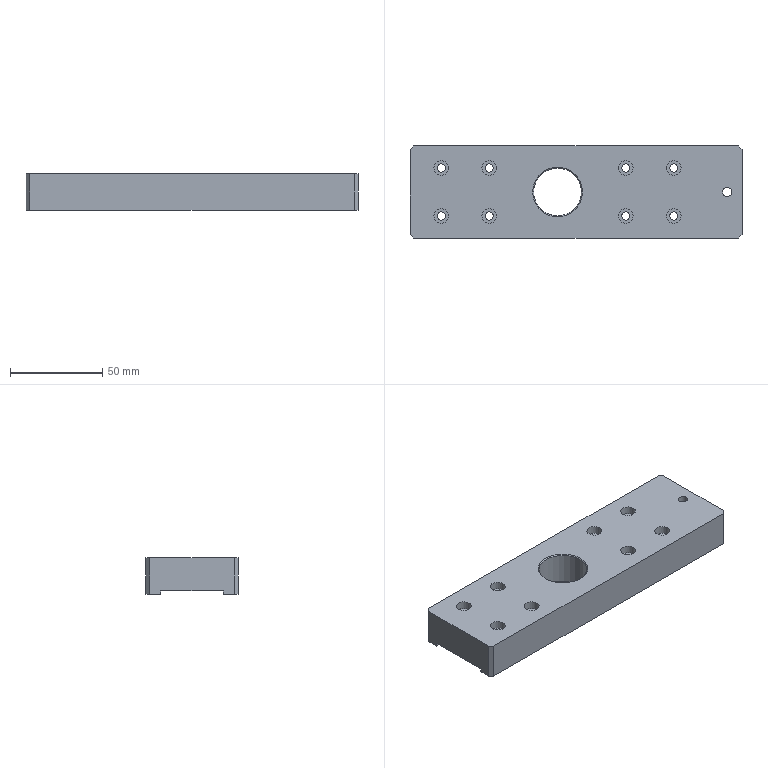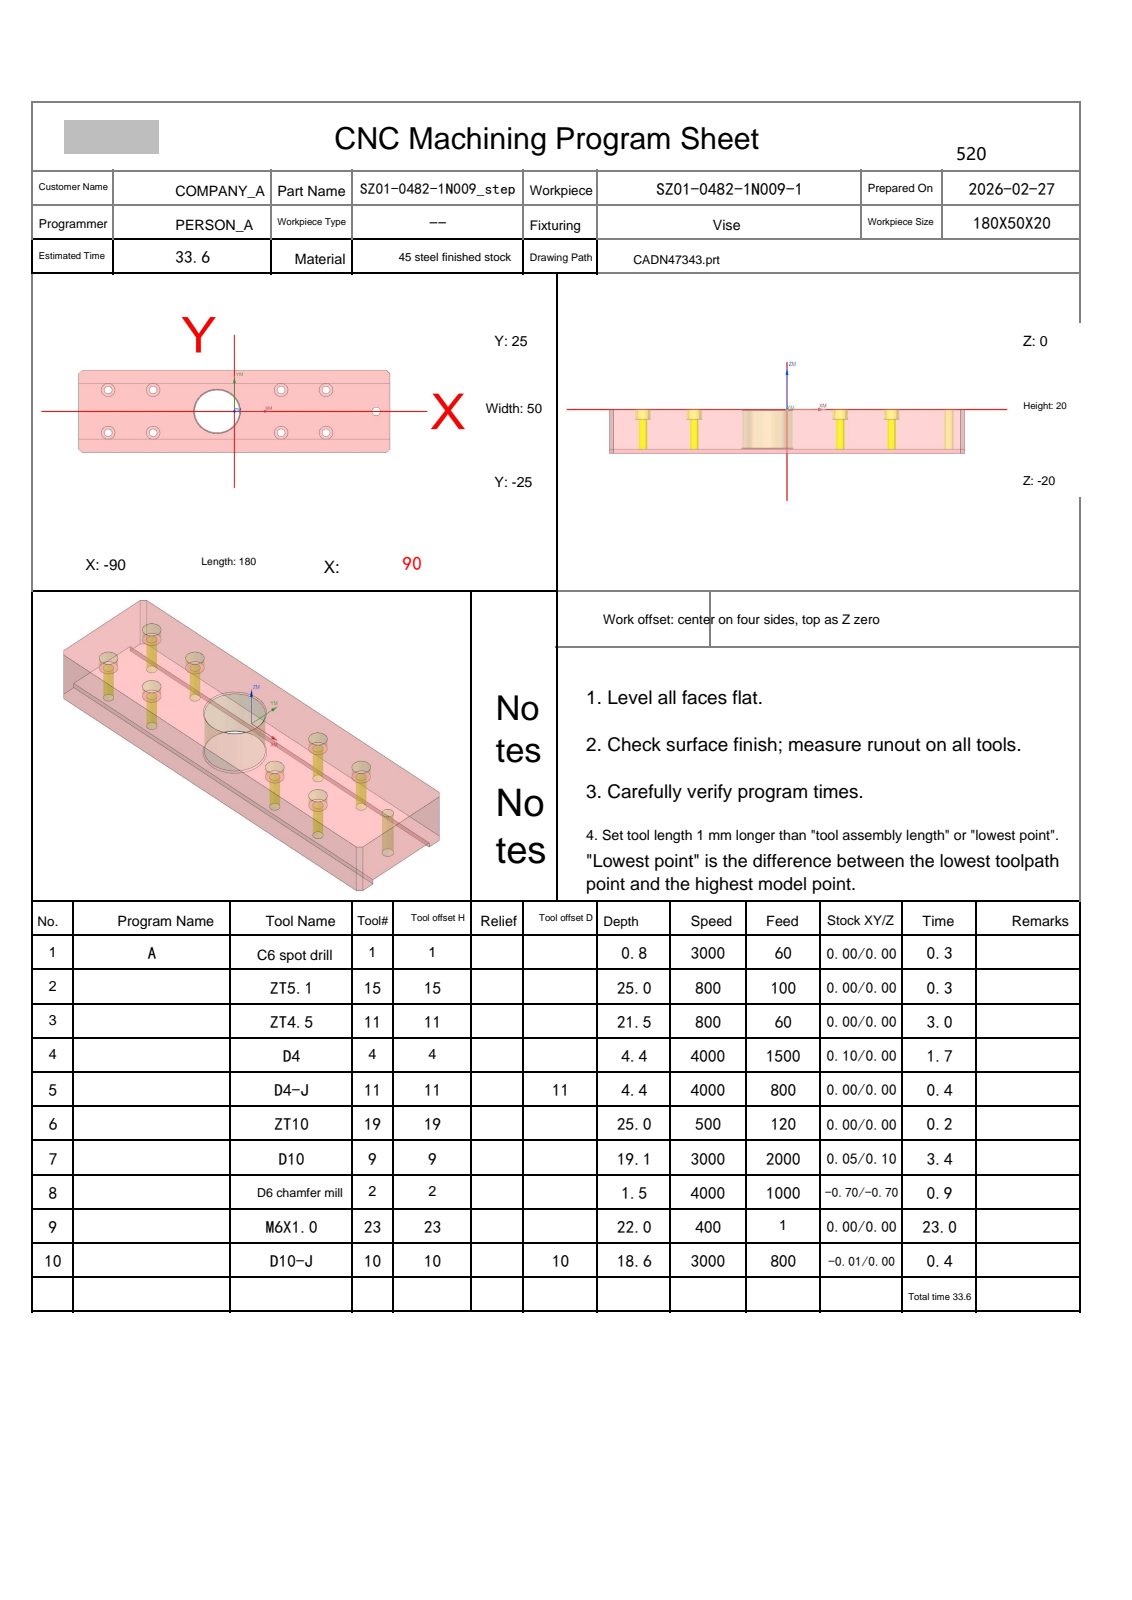NC program | NX | posted by the shop | part box 180 x 50 x 20 mm
Whole program, first 1459 of 1632 lines:
%
O0001
(Machine time: 57.60 MIN)
(===Total Tool:9===)
(T1=C6 spot drill   D=6.   R=0.   D-  H01 Z=-0.8  )
(T15=ZT5.1  D=5.1  DR_a=118 D-  H15 Z=-25.  )
(T11=ZT4.5  D=4.5  DR_a=118 D-  H11 Z=-21.45)
(T4=D4      D=4.   R=0.   D-  H04 Z=-4.4  )
(T19=ZT10   D=10.  DR_a=118 D-  H19 Z=-25.  )
(T9=D10     D=10.  R=0.   D-  H09 Z=-19.1 )
(T2=D6 chamfer mill   D=6.   R=0.   D-  H02 Z=-1.5  )
(T23=M6X1.0 D=5.   DR_a=180 D-  H23 Z=-22.  )
(T10=D10-J  D=10.  R=0.   D10 H10 Z=-18.6 )
G80 G90 G17 G49 G40
G91 G28 Z0
M01
N1 T01 M06
(C6 spot drill  D=6. R=0. H=01 ce=0.00 di=0.00)
T15
G00 G90 G54 X-47. Y13. M03 S3000
G43 H01 Z30.
M08
G98 G81 X-47. Y13. Z-.8 R1. F60.
X-73.
Y-13.
X-47.
X-10. Y0.0
X27. Y-13.
Y13.
X53.
Y-13.
X82. Y0.0
G80
G00 Z30.
G91 G28 Z0.0
M05
M09
G91 G28 Z0.0
M01
N2 T15 M06
(ZT5.1 D=5.1 DR_a=118 H=15)
T11
G00 G90 G54 X82. Y0.0 M03 S800
G43 H15 Z30.
M08
G98 G83 X82. Y0.0 Z-25. R1. F100. Q2.
G80
G00 Z30.
G91 G28 Z0.0
M05
M09
G91 G28 Z0.0
M01
N3 T11 M06
(ZT4.5 D=4.5 DR_a=118 H=11)
T04
G00 G90 G54 X-47. Y-13. M03 S800
G43 H11 Z30.
M08
G98 G83 X-47. Y-13. Z-21.452 R1. F60. Q1.
X-73.
Y13.
X-47.
X27.
Y-13.
X53.
Y13.
G80
G00 Z30.
G91 G28 Z0.0
M05
M09
G91 G28 Z0.0
M01
N4 T04 M06
(D4  D=4. R=0. H=04 ce=0.10 di=0.00)
T11
G00 G90 G54 X-73. Y-13. M03 S4000
G43 H04 Z30.
M08
Z.5
G03 X-72.05 Y-13.95 I.95 J0.0 F1500.
X-71.1 Y-13. I0.0 J.95
X-71.1 Y-13. Z.3 I-1.9 J0.0
X-71.1 Y-13. Z.1 I-1.9 J0.0
X-71.1 Y-13. Z-.1 I-1.9 J0.0
X-71.1 Y-13. Z-.3 I-1.9 J0.0
X-71.1 Y-13. Z-.5 I-1.9 J0.0
X-71.1 Y-13. Z-.7 I-1.9 J0.0
X-71.1 Y-13. Z-.9 I-1.9 J0.0
X-71.1 Y-13. Z-1.1 I-1.9 J0.0
X-71.1 Y-13. Z-1.3 I-1.9 J0.0
X-71.1 Y-13. Z-1.5 I-1.9 J0.0
X-71.1 Y-13. Z-1.7 I-1.9 J0.0
X-71.1 Y-13. Z-1.9 I-1.9 J0.0
X-71.1 Y-13. Z-2.1 I-1.9 J0.0
X-71.1 Y-13. Z-2.3 I-1.9 J0.0
X-71.1 Y-13. Z-2.5 I-1.9 J0.0
X-71.1 Y-13. Z-2.7 I-1.9 J0.0
X-71.1 Y-13. Z-2.9 I-1.9 J0.0
X-71.1 Y-13. Z-3.1 I-1.9 J0.0
X-71.1 Y-13. Z-3.3 I-1.9 J0.0
X-71.1 Y-13. Z-3.5 I-1.9 J0.0
X-71.1 Y-13. Z-3.7 I-1.9 J0.0
X-71.1 Y-13. Z-3.9 I-1.9 J0.0
X-71.1 Y-13. Z-4.1 I-1.9 J0.0
X-71.1 Y-13. Z-4.3 I-1.9 J0.0
X-74.9 Y-13. Z-4.4 I-1.9 J0.0
X-73. Y-14.9 I1.9 J0.0
X-71.1 Y-13. I0.0 J1.9
X-73. Y-11.1 I-1.9 J0.0
X-74.9 Y-13. I0.0 J-1.9
X-73.95 Y-13.95 I.95 J0.0
X-73. Y-13. I0.0 J.95
G00 Z30.
Y13.
Z.5
G03 X-72.05 Y12.05 I.95 J0.0
X-71.1 Y13. I0.0 J.95
X-71.1 Y13. Z.3 I-1.9 J0.0
X-71.1 Y13. Z.1 I-1.9 J0.0
X-71.1 Y13. Z-.1 I-1.9 J0.0
X-71.1 Y13. Z-.3 I-1.9 J0.0
X-71.1 Y13. Z-.5 I-1.9 J0.0
X-71.1 Y13. Z-.7 I-1.9 J0.0
X-71.1 Y13. Z-.9 I-1.9 J0.0
X-71.1 Y13. Z-1.1 I-1.9 J0.0
X-71.1 Y13. Z-1.3 I-1.9 J0.0
X-71.1 Y13. Z-1.5 I-1.9 J0.0
X-71.1 Y13. Z-1.7 I-1.9 J0.0
X-71.1 Y13. Z-1.9 I-1.9 J0.0
X-71.1 Y13. Z-2.1 I-1.9 J0.0
X-71.1 Y13. Z-2.3 I-1.9 J0.0
X-71.1 Y13. Z-2.5 I-1.9 J0.0
X-71.1 Y13. Z-2.7 I-1.9 J0.0
X-71.1 Y13. Z-2.9 I-1.9 J0.0
X-71.1 Y13. Z-3.1 I-1.9 J0.0
X-71.1 Y13. Z-3.3 I-1.9 J0.0
X-71.1 Y13. Z-3.5 I-1.9 J0.0
X-71.1 Y13. Z-3.7 I-1.9 J0.0
X-71.1 Y13. Z-3.9 I-1.9 J0.0
X-71.1 Y13. Z-4.1 I-1.9 J0.0
X-71.1 Y13. Z-4.3 I-1.9 J0.0
X-74.9 Y13. Z-4.4 I-1.9 J0.0
X-73. Y11.1 I1.9 J0.0
X-71.1 Y13. I0.0 J1.9
X-73. Y14.9 I-1.9 J0.0
X-74.9 Y13. I0.0 J-1.9
X-73.95 Y12.05 I.95 J0.0
X-73. Y13. I0.0 J.95
G00 Z30.
X-47.
Z.5
G03 X-46.05 Y12.05 I.95 J0.0
X-45.1 Y13. I0.0 J.95
X-45.1 Y13. Z.3 I-1.9 J0.0
X-45.1 Y13. Z.1 I-1.9 J0.0
X-45.1 Y13. Z-.1 I-1.9 J0.0
X-45.1 Y13. Z-.3 I-1.9 J0.0
X-45.1 Y13. Z-.5 I-1.9 J0.0
X-45.1 Y13. Z-.7 I-1.9 J0.0
X-45.1 Y13. Z-.9 I-1.9 J0.0
X-45.1 Y13. Z-1.1 I-1.9 J0.0
X-45.1 Y13. Z-1.3 I-1.9 J0.0
X-45.1 Y13. Z-1.5 I-1.9 J0.0
X-45.1 Y13. Z-1.7 I-1.9 J0.0
X-45.1 Y13. Z-1.9 I-1.9 J0.0
X-45.1 Y13. Z-2.1 I-1.9 J0.0
X-45.1 Y13. Z-2.3 I-1.9 J0.0
X-45.1 Y13. Z-2.5 I-1.9 J0.0
X-45.1 Y13. Z-2.7 I-1.9 J0.0
X-45.1 Y13. Z-2.9 I-1.9 J0.0
X-45.1 Y13. Z-3.1 I-1.9 J0.0
X-45.1 Y13. Z-3.3 I-1.9 J0.0
X-45.1 Y13. Z-3.5 I-1.9 J0.0
X-45.1 Y13. Z-3.7 I-1.9 J0.0
X-45.1 Y13. Z-3.9 I-1.9 J0.0
X-45.1 Y13. Z-4.1 I-1.9 J0.0
X-45.1 Y13. Z-4.3 I-1.9 J0.0
X-48.9 Y13. Z-4.4 I-1.9 J0.0
X-47. Y11.1 I1.9 J0.0
X-45.1 Y13. I0.0 J1.9
X-47. Y14.9 I-1.9 J0.0
X-48.9 Y13. I0.0 J-1.9
X-47.95 Y12.05 I.95 J0.0
X-47. Y13. I0.0 J.95
G00 Z30.
Y-13.
Z.5
G03 X-46.05 Y-13.95 I.95 J0.0
X-45.1 Y-13. I0.0 J.95
X-45.1 Y-13. Z.3 I-1.9 J0.0
X-45.1 Y-13. Z.1 I-1.9 J0.0
X-45.1 Y-13. Z-.1 I-1.9 J0.0
X-45.1 Y-13. Z-.3 I-1.9 J0.0
X-45.1 Y-13. Z-.5 I-1.9 J0.0
X-45.1 Y-13. Z-.7 I-1.9 J0.0
X-45.1 Y-13. Z-.9 I-1.9 J0.0
X-45.1 Y-13. Z-1.1 I-1.9 J0.0
X-45.1 Y-13. Z-1.3 I-1.9 J0.0
X-45.1 Y-13. Z-1.5 I-1.9 J0.0
X-45.1 Y-13. Z-1.7 I-1.9 J0.0
X-45.1 Y-13. Z-1.9 I-1.9 J0.0
X-45.1 Y-13. Z-2.1 I-1.9 J0.0
X-45.1 Y-13. Z-2.3 I-1.9 J0.0
X-45.1 Y-13. Z-2.5 I-1.9 J0.0
X-45.1 Y-13. Z-2.7 I-1.9 J0.0
X-45.1 Y-13. Z-2.9 I-1.9 J0.0
X-45.1 Y-13. Z-3.1 I-1.9 J0.0
X-45.1 Y-13. Z-3.3 I-1.9 J0.0
X-45.1 Y-13. Z-3.5 I-1.9 J0.0
X-45.1 Y-13. Z-3.7 I-1.9 J0.0
X-45.1 Y-13. Z-3.9 I-1.9 J0.0
X-45.1 Y-13. Z-4.1 I-1.9 J0.0
X-45.1 Y-13. Z-4.3 I-1.9 J0.0
X-48.9 Y-13. Z-4.4 I-1.9 J0.0
X-47. Y-14.9 I1.9 J0.0
X-45.1 Y-13. I0.0 J1.9
X-47. Y-11.1 I-1.9 J0.0
X-48.9 Y-13. I0.0 J-1.9
X-47.95 Y-13.95 I.95 J0.0
X-47. Y-13. I0.0 J.95
G00 Z30.
X27.
Z.5
G03 X27.95 Y-13.95 I.95 J0.0
X28.9 Y-13. I0.0 J.95
X28.9 Y-13. Z.3 I-1.9 J0.0
X28.9 Y-13. Z.1 I-1.9 J0.0
X28.9 Y-13. Z-.1 I-1.9 J0.0
X28.9 Y-13. Z-.3 I-1.9 J0.0
X28.9 Y-13. Z-.5 I-1.9 J0.0
X28.9 Y-13. Z-.7 I-1.9 J0.0
X28.9 Y-13. Z-.9 I-1.9 J0.0
X28.9 Y-13. Z-1.1 I-1.9 J0.0
X28.9 Y-13. Z-1.3 I-1.9 J0.0
X28.9 Y-13. Z-1.5 I-1.9 J0.0
X28.9 Y-13. Z-1.7 I-1.9 J0.0
X28.9 Y-13. Z-1.9 I-1.9 J0.0
X28.9 Y-13. Z-2.1 I-1.9 J0.0
X28.9 Y-13. Z-2.3 I-1.9 J0.0
X28.9 Y-13. Z-2.5 I-1.9 J0.0
X28.9 Y-13. Z-2.7 I-1.9 J0.0
X28.9 Y-13. Z-2.9 I-1.9 J0.0
X28.9 Y-13. Z-3.1 I-1.9 J0.0
X28.9 Y-13. Z-3.3 I-1.9 J0.0
X28.9 Y-13. Z-3.5 I-1.9 J0.0
X28.9 Y-13. Z-3.7 I-1.9 J0.0
X28.9 Y-13. Z-3.9 I-1.9 J0.0
X28.9 Y-13. Z-4.1 I-1.9 J0.0
X28.9 Y-13. Z-4.3 I-1.9 J0.0
X25.1 Y-13. Z-4.4 I-1.9 J0.0
X27. Y-14.9 I1.9 J0.0
X28.9 Y-13. I0.0 J1.9
X27. Y-11.1 I-1.9 J0.0
X25.1 Y-13. I0.0 J-1.9
X26.05 Y-13.95 I.95 J0.0
X27. Y-13. I0.0 J.95
G00 Z30.
X53.
Z.5
G03 X53.95 Y-13.95 I.95 J0.0
X54.9 Y-13. I0.0 J.95
X54.9 Y-13. Z.3 I-1.9 J0.0
X54.9 Y-13. Z.1 I-1.9 J0.0
X54.9 Y-13. Z-.1 I-1.9 J0.0
X54.9 Y-13. Z-.3 I-1.9 J0.0
X54.9 Y-13. Z-.5 I-1.9 J0.0
X54.9 Y-13. Z-.7 I-1.9 J0.0
X54.9 Y-13. Z-.9 I-1.9 J0.0
X54.9 Y-13. Z-1.1 I-1.9 J0.0
X54.9 Y-13. Z-1.3 I-1.9 J0.0
X54.9 Y-13. Z-1.5 I-1.9 J0.0
X54.9 Y-13. Z-1.7 I-1.9 J0.0
X54.9 Y-13. Z-1.9 I-1.9 J0.0
X54.9 Y-13. Z-2.1 I-1.9 J0.0
X54.9 Y-13. Z-2.3 I-1.9 J0.0
X54.9 Y-13. Z-2.5 I-1.9 J0.0
X54.9 Y-13. Z-2.7 I-1.9 J0.0
X54.9 Y-13. Z-2.9 I-1.9 J0.0
X54.9 Y-13. Z-3.1 I-1.9 J0.0
X54.9 Y-13. Z-3.3 I-1.9 J0.0
X54.9 Y-13. Z-3.5 I-1.9 J0.0
X54.9 Y-13. Z-3.7 I-1.9 J0.0
X54.9 Y-13. Z-3.9 I-1.9 J0.0
X54.9 Y-13. Z-4.1 I-1.9 J0.0
X54.9 Y-13. Z-4.3 I-1.9 J0.0
X51.1 Y-13. Z-4.4 I-1.9 J0.0
X53. Y-14.9 I1.9 J0.0
X54.9 Y-13. I0.0 J1.9
X53. Y-11.1 I-1.9 J0.0
X51.1 Y-13. I0.0 J-1.9
X52.05 Y-13.95 I.95 J0.0
X53. Y-13. I0.0 J.95
G00 Z30.
Y13.
Z.5
G03 X53.95 Y12.05 I.95 J0.0
X54.9 Y13. I0.0 J.95
X54.9 Y13. Z.3 I-1.9 J0.0
X54.9 Y13. Z.1 I-1.9 J0.0
X54.9 Y13. Z-.1 I-1.9 J0.0
X54.9 Y13. Z-.3 I-1.9 J0.0
X54.9 Y13. Z-.5 I-1.9 J0.0
X54.9 Y13. Z-.7 I-1.9 J0.0
X54.9 Y13. Z-.9 I-1.9 J0.0
X54.9 Y13. Z-1.1 I-1.9 J0.0
X54.9 Y13. Z-1.3 I-1.9 J0.0
X54.9 Y13. Z-1.5 I-1.9 J0.0
X54.9 Y13. Z-1.7 I-1.9 J0.0
X54.9 Y13. Z-1.9 I-1.9 J0.0
X54.9 Y13. Z-2.1 I-1.9 J0.0
X54.9 Y13. Z-2.3 I-1.9 J0.0
X54.9 Y13. Z-2.5 I-1.9 J0.0
X54.9 Y13. Z-2.7 I-1.9 J0.0
X54.9 Y13. Z-2.9 I-1.9 J0.0
X54.9 Y13. Z-3.1 I-1.9 J0.0
X54.9 Y13. Z-3.3 I-1.9 J0.0
X54.9 Y13. Z-3.5 I-1.9 J0.0
X54.9 Y13. Z-3.7 I-1.9 J0.0
X54.9 Y13. Z-3.9 I-1.9 J0.0
X54.9 Y13. Z-4.1 I-1.9 J0.0
X54.9 Y13. Z-4.3 I-1.9 J0.0
X51.1 Y13. Z-4.4 I-1.9 J0.0
X53. Y11.1 I1.9 J0.0
X54.9 Y13. I0.0 J1.9
X53. Y14.9 I-1.9 J0.0
X51.1 Y13. I0.0 J-1.9
X52.05 Y12.05 I.95 J0.0
X53. Y13. I0.0 J.95
G00 Z30.
X27.
Z.5
G03 X27.95 Y12.05 I.95 J0.0
X28.9 Y13. I0.0 J.95
X28.9 Y13. Z.3 I-1.9 J0.0
X28.9 Y13. Z.1 I-1.9 J0.0
X28.9 Y13. Z-.1 I-1.9 J0.0
X28.9 Y13. Z-.3 I-1.9 J0.0
X28.9 Y13. Z-.5 I-1.9 J0.0
X28.9 Y13. Z-.7 I-1.9 J0.0
X28.9 Y13. Z-.9 I-1.9 J0.0
X28.9 Y13. Z-1.1 I-1.9 J0.0
X28.9 Y13. Z-1.3 I-1.9 J0.0
X28.9 Y13. Z-1.5 I-1.9 J0.0
X28.9 Y13. Z-1.7 I-1.9 J0.0
X28.9 Y13. Z-1.9 I-1.9 J0.0
X28.9 Y13. Z-2.1 I-1.9 J0.0
X28.9 Y13. Z-2.3 I-1.9 J0.0
X28.9 Y13. Z-2.5 I-1.9 J0.0
X28.9 Y13. Z-2.7 I-1.9 J0.0
X28.9 Y13. Z-2.9 I-1.9 J0.0
X28.9 Y13. Z-3.1 I-1.9 J0.0
X28.9 Y13. Z-3.3 I-1.9 J0.0
X28.9 Y13. Z-3.5 I-1.9 J0.0
X28.9 Y13. Z-3.7 I-1.9 J0.0
X28.9 Y13. Z-3.9 I-1.9 J0.0
X28.9 Y13. Z-4.1 I-1.9 J0.0
X28.9 Y13. Z-4.3 I-1.9 J0.0
X25.1 Y13. Z-4.4 I-1.9 J0.0
X27. Y11.1 I1.9 J0.0
X28.9 Y13. I0.0 J1.9
X27. Y14.9 I-1.9 J0.0
X25.1 Y13. I0.0 J-1.9
X26.05 Y12.05 I.95 J0.0
X27. Y13. I0.0 J.95
G00 Z30.
G91 G28 Z0.0
M05
M09
G91 G28 Z0.0
M01
N5 T11 M06
(D4-J  D=4. R=0. H=11 ce=0.00 di=0.00)
T19
G00 G90 G54 X-73. Y-13. M03 S4000
G43 H11 Z30.
M08
Z.5
G41 D11
G01 X-72.96 Y-13.196 F800.
G03 X-71.99 Y-13.99 I.97 J.196
X-71. Y-13. I0.0 J.99
X-71.016 Y-13.251 Z-4.4 I-2. J0.0
X-71. Y-13. I-1.984 J.251
X-73. Y-11. I-2. J0.0
X-75. Y-13. I0.0 J-2.
X-73. Y-15. I2. J0.0
X-71.016 Y-13.251 I0.0 J2.
G01 X-71.008 Y-13.127
G03 X-71.998 Y-12.137 I-.99 J0.0
X-72.936 Y-12.81 I0.0 J-.99
G01 G40 X-73. Y-13.
G00 Z30.
Y13.
Z.5
G41 D11
G01 X-72.96 Y12.804
G03 X-71.99 Y12.01 I.97 J.196
X-71. Y13. I0.0 J.99
X-71.016 Y12.749 Z-4.4 I-2. J0.0
X-71. Y13. I-1.984 J.251
X-73. Y15. I-2. J0.0
X-75. Y13. I0.0 J-2.
X-73. Y11. I2. J0.0
X-71.016 Y12.749 I0.0 J2.
G01 X-71.008 Y12.873
G03 X-71.998 Y13.863 I-.99 J0.0
X-72.936 Y13.19 I0.0 J-.99
G01 G40 X-73. Y13.
G00 Z30.
X-47.
Z.5
G41 D11
G01 X-46.96 Y12.804
G03 X-45.99 Y12.01 I.97 J.196
X-45. Y13. I0.0 J.99
X-45.016 Y12.749 Z-4.4 I-2. J0.0
X-45. Y13. I-1.984 J.251
X-47. Y15. I-2. J0.0
X-49. Y13. I0.0 J-2.
X-47. Y11. I2. J0.0
X-45.016 Y12.749 I0.0 J2.
G01 X-45.008 Y12.873
G03 X-45.998 Y13.863 I-.99 J0.0
X-46.936 Y13.19 I0.0 J-.99
G01 G40 X-47. Y13.
G00 Z30.
Y-13.
Z.5
G41 D11
G01 X-46.96 Y-13.196
G03 X-45.99 Y-13.99 I.97 J.196
X-45. Y-13. I0.0 J.99
X-45.016 Y-13.251 Z-4.4 I-2. J0.0
X-45. Y-13. I-1.984 J.251
X-47. Y-11. I-2. J0.0
X-49. Y-13. I0.0 J-2.
X-47. Y-15. I2. J0.0
X-45.016 Y-13.251 I0.0 J2.
G01 X-45.008 Y-13.127
G03 X-45.998 Y-12.137 I-.99 J0.0
X-46.936 Y-12.81 I0.0 J-.99
G01 G40 X-47. Y-13.
G00 Z30.
X27.
Z.5
G41 D11
G01 X27.04 Y-13.196
G03 X28.01 Y-13.99 I.97 J.196
X29. Y-13. I0.0 J.99
X28.984 Y-13.251 Z-4.4 I-2. J0.0
X29. Y-13. I-1.984 J.251
X27. Y-11. I-2. J0.0
X25. Y-13. I0.0 J-2.
X27. Y-15. I2. J0.0
X28.984 Y-13.251 I0.0 J2.
G01 X28.992 Y-13.127
G03 X28.002 Y-12.137 I-.99 J0.0
X27.064 Y-12.81 I0.0 J-.99
G01 G40 X27. Y-13.
G00 Z30.
X53.
Z.5
G41 D11
G01 X53.04 Y-13.196
G03 X54.01 Y-13.99 I.97 J.196
X55. Y-13. I0.0 J.99
X54.984 Y-13.251 Z-4.4 I-2. J0.0
X55. Y-13. I-1.984 J.251
X53. Y-11. I-2. J0.0
X51. Y-13. I0.0 J-2.
X53. Y-15. I2. J0.0
X54.984 Y-13.251 I0.0 J2.
G01 X54.992 Y-13.127
G03 X54.002 Y-12.137 I-.99 J0.0
X53.064 Y-12.81 I0.0 J-.99
G01 G40 X53. Y-13.
G00 Z30.
Y13.
Z.5
G41 D11
G01 X53.04 Y12.804
G03 X54.01 Y12.01 I.97 J.196
X55. Y13. I0.0 J.99
X54.984 Y12.749 Z-4.4 I-2. J0.0
X55. Y13. I-1.984 J.251
X53. Y15. I-2. J0.0
X51. Y13. I0.0 J-2.
X53. Y11. I2. J0.0
X54.984 Y12.749 I0.0 J2.
G01 X54.992 Y12.873
G03 X54.002 Y13.863 I-.99 J0.0
X53.064 Y13.19 I0.0 J-.99
G01 G40 X53. Y13.
G00 Z30.
X27.
Z.5
G41 D11
G01 X27.04 Y12.804
G03 X28.01 Y12.01 I.97 J.196
X29. Y13. I0.0 J.99
X28.984 Y12.749 Z-4.4 I-2. J0.0
X29. Y13. I-1.984 J.251
X27. Y15. I-2. J0.0
X25. Y13. I0.0 J-2.
X27. Y11. I2. J0.0
X28.984 Y12.749 I0.0 J2.
G01 X28.992 Y12.873
G03 X28.002 Y13.863 I-.99 J0.0
X27.064 Y13.19 I0.0 J-.99
G01 G40 X27. Y13.
G00 Z30.
G91 G28 Z0.0
M05
M09
G91 G28 Z0.0
M01
N6 T19 M06
(ZT10 D=10. DR_a=118 H=19)
T09
G00 G90 G54 X-10. Y0.0 M03 S500
G43 H19 Z30.
M08
G98 G83 X-10. Y0.0 Z-25. R1. F120. Q2.
G80
G00 Z30.
G91 G28 Z0.0
M05
M09
G91 G28 Z0.0
M01
N7 T09 M06
(D10  D=10. R=0. H=09 ce=0.10 di=0.10)
T02
G00 G90 G54 X85.242 Y34.97 M03 S3000
G43 H09 Z30.
M08
Z-.5
G01 X91.606 Y28.606 F2000.
X93.606 Y26.606
X99.97 Y20.242
G00 Z-1.
G01 X93.606 Y26.606
X91.606 Y28.606
X85.242 Y34.97
G00 Z-1.5
G01 X91.606 Y28.606
X93.606 Y26.606
X99.97 Y20.242
G00 Z-2.
G01 X93.606 Y26.606
X91.606 Y28.606
X85.242 Y34.97
G00 Z-2.5
G01 X91.606 Y28.606
X93.606 Y26.606
X99.97 Y20.242
G00 Z-3.
G01 X93.606 Y26.606
X91.606 Y28.606
X85.242 Y34.97
G00 Z-3.5
G01 X91.606 Y28.606
X93.606 Y26.606
X99.97 Y20.242
G00 Z-4.
G01 X93.606 Y26.606
X91.606 Y28.606
X85.242 Y34.97
G00 Z-4.5
G01 X91.606 Y28.606
X93.606 Y26.606
X99.97 Y20.242
G00 Z-5.
G01 X93.606 Y26.606
X91.606 Y28.606
X85.242 Y34.97
G00 Z-5.5
G01 X91.606 Y28.606
X93.606 Y26.606
X99.97 Y20.242
G00 Z-6.
G01 X93.606 Y26.606
X91.606 Y28.606
X85.242 Y34.97
G00 Z-6.5
G01 X91.606 Y28.606
X93.606 Y26.606
X99.97 Y20.242
G00 Z-7.
G01 X93.606 Y26.606
X91.606 Y28.606
X85.242 Y34.97
G00 Z-7.5
G01 X91.606 Y28.606
X93.606 Y26.606
X99.97 Y20.242
G00 Z-8.
G01 X93.606 Y26.606
X91.606 Y28.606
X85.242 Y34.97
G00 Z-8.5
G01 X91.606 Y28.606
X93.606 Y26.606
X99.97 Y20.242
G00 Z-9.
G01 X93.606 Y26.606
X91.606 Y28.606
X85.242 Y34.97
G00 Z-9.5
G01 X91.606 Y28.606
X93.606 Y26.606
X99.97 Y20.242
G00 Z-10.
G01 X93.606 Y26.606
X91.606 Y28.606
X85.242 Y34.97
G00 Z-10.5
G01 X91.606 Y28.606
X93.606 Y26.606
X99.97 Y20.242
G00 Z-10.9
G01 X93.606 Y26.606
X91.606 Y28.606
X85.242 Y34.97
G00 Z30.
X99.97 Y-20.242
Z-.5
G01 X93.606 Y-26.606
X91.606 Y-28.606
X85.242 Y-34.97
G00 Z-1.
G01 X91.606 Y-28.606
X93.606 Y-26.606
X99.97 Y-20.242
G00 Z-1.5
G01 X93.606 Y-26.606
X91.606 Y-28.606
X85.242 Y-34.97
G00 Z-2.
G01 X91.606 Y-28.606
X93.606 Y-26.606
X99.97 Y-20.242
G00 Z-2.5
G01 X93.606 Y-26.606
X91.606 Y-28.606
X85.242 Y-34.97
G00 Z-3.
G01 X91.606 Y-28.606
X93.606 Y-26.606
X99.97 Y-20.242
G00 Z-3.5
G01 X93.606 Y-26.606
X91.606 Y-28.606
X85.242 Y-34.97
G00 Z-4.
G01 X91.606 Y-28.606
X93.606 Y-26.606
X99.97 Y-20.242
G00 Z-4.5
G01 X93.606 Y-26.606
X91.606 Y-28.606
X85.242 Y-34.97
G00 Z-5.
G01 X91.606 Y-28.606
X93.606 Y-26.606
X99.97 Y-20.242
G00 Z-5.5
G01 X93.606 Y-26.606
X91.606 Y-28.606
X85.242 Y-34.97
G00 Z-6.
G01 X91.606 Y-28.606
X93.606 Y-26.606
X99.97 Y-20.242
G00 Z-6.5
G01 X93.606 Y-26.606
X91.606 Y-28.606
X85.242 Y-34.97
G00 Z-7.
G01 X91.606 Y-28.606
X93.606 Y-26.606
X99.97 Y-20.242
G00 Z-7.5
G01 X93.606 Y-26.606
X91.606 Y-28.606
X85.242 Y-34.97
G00 Z-8.
G01 X91.606 Y-28.606
X93.606 Y-26.606
X99.97 Y-20.242
G00 Z-8.5
G01 X93.606 Y-26.606
X91.606 Y-28.606
X85.242 Y-34.97
G00 Z-9.
G01 X91.606 Y-28.606
X93.606 Y-26.606
X99.97 Y-20.242
G00 Z-9.5
G01 X93.606 Y-26.606
X91.606 Y-28.606
X85.242 Y-34.97
G00 Z-10.
G01 X91.606 Y-28.606
X93.606 Y-26.606
X99.97 Y-20.242
G00 Z-10.5
G01 X93.606 Y-26.606
X91.606 Y-28.606
X85.242 Y-34.97
G00 Z-10.9
G01 X91.606 Y-28.606
X93.606 Y-26.606
X99.97 Y-20.242
G00 Z30.
X-85.242 Y-34.97
Z-.5
G01 X-91.606 Y-28.606
X-93.606 Y-26.606
X-99.97 Y-20.242
G00 Z-1.
G01 X-93.606 Y-26.606
X-91.606 Y-28.606
X-85.242 Y-34.97
G00 Z-1.5
G01 X-91.606 Y-28.606
X-93.606 Y-26.606
X-99.97 Y-20.242
G00 Z-2.
G01 X-93.606 Y-26.606
X-91.606 Y-28.606
X-85.242 Y-34.97
G00 Z-2.5
G01 X-91.606 Y-28.606
X-93.606 Y-26.606
X-99.97 Y-20.242
G00 Z-3.
G01 X-93.606 Y-26.606
X-91.606 Y-28.606
X-85.242 Y-34.97
G00 Z-3.5
G01 X-91.606 Y-28.606
X-93.606 Y-26.606
X-99.97 Y-20.242
G00 Z-4.
G01 X-93.606 Y-26.606
X-91.606 Y-28.606
X-85.242 Y-34.97
G00 Z-4.5
G01 X-91.606 Y-28.606
X-93.606 Y-26.606
X-99.97 Y-20.242
G00 Z-5.
G01 X-93.606 Y-26.606
X-91.606 Y-28.606
X-85.242 Y-34.97
G00 Z-5.5
G01 X-91.606 Y-28.606
X-93.606 Y-26.606
X-99.97 Y-20.242
G00 Z-6.
G01 X-93.606 Y-26.606
X-91.606 Y-28.606
X-85.242 Y-34.97
G00 Z-6.5
G01 X-91.606 Y-28.606
X-93.606 Y-26.606
X-99.97 Y-20.242
G00 Z-7.
G01 X-93.606 Y-26.606
X-91.606 Y-28.606
X-85.242 Y-34.97
G00 Z-7.5
G01 X-91.606 Y-28.606
X-93.606 Y-26.606
X-99.97 Y-20.242
G00 Z-8.
G01 X-93.606 Y-26.606
X-91.606 Y-28.606
X-85.242 Y-34.97
G00 Z-8.5
G01 X-91.606 Y-28.606
X-93.606 Y-26.606
X-99.97 Y-20.242
G00 Z-9.
G01 X-93.606 Y-26.606
X-91.606 Y-28.606
X-85.242 Y-34.97
G00 Z-9.5
G01 X-91.606 Y-28.606
X-93.606 Y-26.606
X-99.97 Y-20.242
G00 Z-10.
G01 X-93.606 Y-26.606
X-91.606 Y-28.606
X-85.242 Y-34.97
G00 Z-10.5
G01 X-91.606 Y-28.606
X-93.606 Y-26.606
X-99.97 Y-20.242
G00 Z-10.9
G01 X-93.606 Y-26.606
X-91.606 Y-28.606
X-85.242 Y-34.97
G00 Z30.
X-99.97 Y20.242
Z-.5
G01 X-93.606 Y26.606
X-91.606 Y28.606
X-85.242 Y34.97
G00 Z-1.
G01 X-91.606 Y28.606
X-93.606 Y26.606
X-99.97 Y20.242
G00 Z-1.5
G01 X-93.606 Y26.606
X-91.606 Y28.606
X-85.242 Y34.97
G00 Z-2.
G01 X-91.606 Y28.606
X-93.606 Y26.606
X-99.97 Y20.242
G00 Z-2.5
G01 X-93.606 Y26.606
X-91.606 Y28.606
X-85.242 Y34.97
G00 Z-3.
G01 X-91.606 Y28.606
X-93.606 Y26.606
X-99.97 Y20.242
G00 Z-3.5
G01 X-93.606 Y26.606
X-91.606 Y28.606
X-85.242 Y34.97
G00 Z-4.
G01 X-91.606 Y28.606
X-93.606 Y26.606
X-99.97 Y20.242
G00 Z-4.5
G01 X-93.606 Y26.606
X-91.606 Y28.606
X-85.242 Y34.97
G00 Z-5.
G01 X-91.606 Y28.606
X-93.606 Y26.606
X-99.97 Y20.242
G00 Z-5.5
G01 X-93.606 Y26.606
X-91.606 Y28.606
X-85.242 Y34.97
G00 Z-6.
G01 X-91.606 Y28.606
X-93.606 Y26.606
X-99.97 Y20.242
G00 Z-6.5
G01 X-93.606 Y26.606
X-91.606 Y28.606
X-85.242 Y34.97
G00 Z-7.
G01 X-91.606 Y28.606
X-93.606 Y26.606
X-99.97 Y20.242
G00 Z-7.5
G01 X-93.606 Y26.606
X-91.606 Y28.606
X-85.242 Y34.97
G00 Z-8.
G01 X-91.606 Y28.606
X-93.606 Y26.606
X-99.97 Y20.242
G00 Z-8.5
G01 X-93.606 Y26.606
X-91.606 Y28.606
X-85.242 Y34.97
G00 Z-9.
G01 X-91.606 Y28.606
X-93.606 Y26.606
X-99.97 Y20.242
G00 Z-9.5
G01 X-93.606 Y26.606
X-91.606 Y28.606
X-85.242 Y34.97
G00 Z-10.
G01 X-91.606 Y28.606
X-93.606 Y26.606
X-99.97 Y20.242
G00 Z-10.5
G01 X-93.606 Y26.606
X-91.606 Y28.606
X-85.242 Y34.97
G00 Z-10.9
G01 X-91.606 Y28.606
X-93.606 Y26.606
X-99.97 Y20.242
G00 Z30.
G00 G90 X-15.392 Y5.841 M03 S3000
Z30.
Z1.
G01 X-15.643 Y5.643 Z.983 F2000.
X-16.793 Y4.188 Z.886
X-17.576 Y2.507 Z.789
X-17.95 Y.691 Z.692
Y-.691 Z.619
X-17.576 Y-2.507 Z.522
X-16.793 Y-4.188 Z.425
X-15.643 Y-5.643 Z.328
X-14.188 Y-6.793 Z.231
X-12.507 Y-7.576 Z.133
X-10.691 Y-7.95 Z.036
X-10. Z0.0
G03 X-2.05 Y0.0 Z-.05 I0.0 J7.95
X-10. Y7.95 Z-.099 I-7.95 J0.0
X-17.95 Y0.0 Z-.149 I0.0 J-7.95
X-10. Y-7.95 Z-.199 I7.95 J0.0
X-2.05 Y0.0 Z-.249 I0.0 J7.95
X-10. Y7.95 Z-.298 I-7.95 J0.0
X-17.95 Y0.0 Z-.348 I0.0 J-7.95
X-10. Y-7.95 Z-.398 I7.95 J0.0
X-2.05 Y0.0 Z-.448 I0.0 J7.95
X-10. Y7.95 Z-.497 I-7.95 J0.0
X-17.95 Y0.0 Z-.547 I0.0 J-7.95
X-10. Y-7.95 Z-.597 I7.95 J0.0
X-2.05 Y0.0 Z-.647 I0.0 J7.95
X-10. Y7.95 Z-.696 I-7.95 J0.0
X-17.95 Y0.0 Z-.746 I0.0 J-7.95
X-10. Y-7.95 Z-.796 I7.95 J0.0
X-2.05 Y0.0 Z-.846 I0.0 J7.95
X-10. Y7.95 Z-.895 I-7.95 J0.0
X-17.95 Y0.0 Z-.945 I0.0 J-7.95
X-10. Y-7.95 Z-.995 I7.95 J0.0
X-2.05 Y0.0 Z-1.045 I0.0 J7.95
X-10. Y7.95 Z-1.094 I-7.95 J0.0
X-17.95 Y0.0 Z-1.144 I0.0 J-7.95
X-10. Y-7.95 Z-1.194 I7.95 J0.0
X-2.05 Y0.0 Z-1.243 I0.0 J7.95
X-10. Y7.95 Z-1.293 I-7.95 J0.0
X-17.95 Y0.0 Z-1.343 I0.0 J-7.95
X-10. Y-7.95 Z-1.393 I7.95 J0.0
X-2.05 Y0.0 Z-1.442 I0.0 J7.95
X-10. Y7.95 Z-1.492 I-7.95 J0.0
X-17.95 Y0.0 Z-1.542 I0.0 J-7.95
X-10. Y-7.95 Z-1.592 I7.95 J0.0
X-2.05 Y0.0 Z-1.641 I0.0 J7.95
X-10. Y7.95 Z-1.691 I-7.95 J0.0
X-17.95 Y0.0 Z-1.741 I0.0 J-7.95
X-10. Y-7.95 Z-1.791 I7.95 J0.0
X-2.05 Y0.0 Z-1.84 I0.0 J7.95
X-10. Y7.95 Z-1.89 I-7.95 J0.0
X-17.95 Y0.0 Z-1.94 I0.0 J-7.95
X-10. Y-7.95 Z-1.99 I7.95 J0.0
X-2.05 Y0.0 Z-2.039 I0.0 J7.95
X-10. Y7.95 Z-2.089 I-7.95 J0.0
X-17.95 Y0.0 Z-2.139 I0.0 J-7.95
X-10. Y-7.95 Z-2.189 I7.95 J0.0
X-2.05 Y0.0 Z-2.238 I0.0 J7.95
X-10. Y7.95 Z-2.288 I-7.95 J0.0
X-17.95 Y0.0 Z-2.338 I0.0 J-7.95
X-10. Y-7.95 Z-2.388 I7.95 J0.0
X-2.05 Y0.0 Z-2.437 I0.0 J7.95
X-10. Y7.95 Z-2.487 I-7.95 J0.0
X-17.95 Y0.0 Z-2.537 I0.0 J-7.95
X-10. Y-7.95 Z-2.586 I7.95 J0.0
X-2.05 Y0.0 Z-2.636 I0.0 J7.95
X-10. Y7.95 Z-2.686 I-7.95 J0.0
X-17.95 Y0.0 Z-2.736 I0.0 J-7.95
X-10. Y-7.95 Z-2.785 I7.95 J0.0
X-2.05 Y0.0 Z-2.835 I0.0 J7.95
X-10. Y7.95 Z-2.885 I-7.95 J0.0
X-17.95 Y0.0 Z-2.935 I0.0 J-7.95
X-10. Y-7.95 Z-2.984 I7.95 J0.0
X-2.05 Y0.0 Z-3.034 I0.0 J7.95
X-10. Y7.95 Z-3.084 I-7.95 J0.0
X-17.95 Y0.0 Z-3.134 I0.0 J-7.95
X-10. Y-7.95 Z-3.183 I7.95 J0.0
X-2.05 Y0.0 Z-3.233 I0.0 J7.95
X-10. Y7.95 Z-3.283 I-7.95 J0.0
X-17.95 Y0.0 Z-3.333 I0.0 J-7.95
X-10. Y-7.95 Z-3.382 I7.95 J0.0
X-2.05 Y0.0 Z-3.432 I0.0 J7.95
X-10. Y7.95 Z-3.482 I-7.95 J0.0
X-17.95 Y0.0 Z-3.532 I0.0 J-7.95
X-10. Y-7.95 Z-3.581 I7.95 J0.0
X-2.05 Y0.0 Z-3.631 I0.0 J7.95
X-10. Y7.95 Z-3.681 I-7.95 J0.0
X-17.95 Y0.0 Z-3.73 I0.0 J-7.95
X-10. Y-7.95 Z-3.78 I7.95 J0.0
X-2.05 Y0.0 Z-3.83 I0.0 J7.95
X-10. Y7.95 Z-3.88 I-7.95 J0.0
X-17.95 Y0.0 Z-3.929 I0.0 J-7.95
X-10. Y-7.95 Z-3.979 I7.95 J0.0
X-2.05 Y0.0 Z-4.029 I0.0 J7.95
X-10. Y7.95 Z-4.079 I-7.95 J0.0
X-17.95 Y0.0 Z-4.128 I0.0 J-7.95
X-10. Y-7.95 Z-4.178 I7.95 J0.0
X-2.05 Y0.0 Z-4.228 I0.0 J7.95
X-10. Y7.95 Z-4.278 I-7.95 J0.0
X-17.95 Y0.0 Z-4.327 I0.0 J-7.95
X-10. Y-7.95 Z-4.377 I7.95 J0.0
X-2.05 Y0.0 Z-4.427 I0.0 J7.95
X-10. Y7.95 Z-4.477 I-7.95 J0.0
X-17.95 Y0.0 Z-4.526 I0.0 J-7.95
X-10. Y-7.95 Z-4.576 I7.95 J0.0
X-2.05 Y0.0 Z-4.626 I0.0 J7.95
X-10. Y7.95 Z-4.676 I-7.95 J0.0
X-17.95 Y0.0 Z-4.725 I0.0 J-7.95
X-10. Y-7.95 Z-4.775 I7.95 J0.0
X-2.05 Y0.0 Z-4.825 I0.0 J7.95
X-10. Y7.95 Z-4.874 I-7.95 J0.0
X-17.95 Y0.0 Z-4.924 I0.0 J-7.95
X-10. Y-7.95 Z-4.974 I7.95 J0.0
X-2.05 Y0.0 Z-5.024 I0.0 J7.95
X-10. Y7.95 Z-5.073 I-7.95 J0.0
X-17.95 Y0.0 Z-5.123 I0.0 J-7.95
X-10. Y-7.95 Z-5.173 I7.95 J0.0
X-2.05 Y0.0 Z-5.223 I0.0 J7.95
X-10. Y7.95 Z-5.272 I-7.95 J0.0
X-17.95 Y0.0 Z-5.322 I0.0 J-7.95
X-10. Y-7.95 Z-5.372 I7.95 J0.0
X-2.05 Y0.0 Z-5.422 I0.0 J7.95
X-10. Y7.95 Z-5.471 I-7.95 J0.0
X-17.95 Y0.0 Z-5.521 I0.0 J-7.95
X-10. Y-7.95 Z-5.571 I7.95 J0.0
X-2.05 Y0.0 Z-5.621 I0.0 J7.95
X-10. Y7.95 Z-5.67 I-7.95 J0.0
X-17.95 Y0.0 Z-5.72 I0.0 J-7.95
X-10. Y-7.95 Z-5.77 I7.95 J0.0
X-2.05 Y0.0 Z-5.82 I0.0 J7.95
X-10. Y7.95 Z-5.869 I-7.95 J0.0
X-17.95 Y0.0 Z-5.919 I0.0 J-7.95
X-10. Y-7.95 Z-5.969 I7.95 J0.0
X-2.05 Y0.0 Z-6.018 I0.0 J7.95
X-10. Y7.95 Z-6.068 I-7.95 J0.0
X-17.95 Y0.0 Z-6.118 I0.0 J-7.95
X-10. Y-7.95 Z-6.168 I7.95 J0.0
X-2.05 Y0.0 Z-6.217 I0.0 J7.95
X-10. Y7.95 Z-6.267 I-7.95 J0.0
X-17.95 Y0.0 Z-6.317 I0.0 J-7.95
X-10. Y-7.95 Z-6.367 I7.95 J0.0
X-2.05 Y0.0 Z-6.416 I0.0 J7.95
X-10. Y7.95 Z-6.466 I-7.95 J0.0
X-17.95 Y0.0 Z-6.516 I0.0 J-7.95
X-10. Y-7.95 Z-6.566 I7.95 J0.0
X-2.05 Y0.0 Z-6.615 I0.0 J7.95
X-10. Y7.95 Z-6.665 I-7.95 J0.0
X-17.95 Y0.0 Z-6.715 I0.0 J-7.95
X-10. Y-7.95 Z-6.765 I7.95 J0.0
X-2.05 Y0.0 Z-6.814 I0.0 J7.95
X-10. Y7.95 Z-6.864 I-7.95 J0.0
X-17.95 Y0.0 Z-6.914 I0.0 J-7.95
X-10. Y-7.95 Z-6.964 I7.95 J0.0
X-2.05 Y0.0 Z-7.013 I0.0 J7.95
X-10. Y7.95 Z-7.063 I-7.95 J0.0
X-17.95 Y0.0 Z-7.113 I0.0 J-7.95
X-10. Y-7.95 Z-7.163 I7.95 J0.0
X-2.05 Y0.0 Z-7.212 I0.0 J7.95
X-10. Y7.95 Z-7.262 I-7.95 J0.0
X-17.95 Y0.0 Z-7.312 I0.0 J-7.95
X-10. Y-7.95 Z-7.361 I7.95 J0.0
X-2.05 Y0.0 Z-7.411 I0.0 J7.95
X-10. Y7.95 Z-7.461 I-7.95 J0.0
X-17.95 Y0.0 Z-7.511 I0.0 J-7.95
X-10. Y-7.95 Z-7.56 I7.95 J0.0
X-2.05 Y0.0 Z-7.61 I0.0 J7.95
X-10. Y7.95 Z-7.66 I-7.95 J0.0
X-17.95 Y0.0 Z-7.71 I0.0 J-7.95
X-10. Y-7.95 Z-7.759 I7.95 J0.0
X-2.05 Y0.0 Z-7.809 I0.0 J7.95
X-10. Y7.95 Z-7.859 I-7.95 J0.0
X-17.95 Y0.0 Z-7.909 I0.0 J-7.95
X-10. Y-7.95 Z-7.958 I7.95 J0.0
X-2.05 Y0.0 Z-8.008 I0.0 J7.95
X-10. Y7.95 Z-8.058 I-7.95 J0.0
X-17.95 Y0.0 Z-8.108 I0.0 J-7.95
X-10. Y-7.95 Z-8.157 I7.95 J0.0
X-2.05 Y0.0 Z-8.207 I0.0 J7.95
X-10. Y7.95 Z-8.257 I-7.95 J0.0
X-17.95 Y0.0 Z-8.307 I0.0 J-7.95
X-10. Y-7.95 Z-8.356 I7.95 J0.0
X-2.05 Y0.0 Z-8.406 I0.0 J7.95
X-10. Y7.95 Z-8.456 I-7.95 J0.0
X-17.95 Y0.0 Z-8.505 I0.0 J-7.95
X-10. Y-7.95 Z-8.555 I7.95 J0.0
X-2.05 Y0.0 Z-8.605 I0.0 J7.95
X-10. Y7.95 Z-8.655 I-7.95 J0.0
X-17.95 Y0.0 Z-8.704 I0.0 J-7.95
X-10. Y-7.95 Z-8.754 I7.95 J0.0
X-2.05 Y0.0 Z-8.804 I0.0 J7.95
X-10. Y7.95 Z-8.854 I-7.95 J0.0
X-17.95 Y0.0 Z-8.903 I0.0 J-7.95
X-10. Y-7.95 Z-8.953 I7.95 J0.0
X-2.05 Y0.0 Z-9.003 I0.0 J7.95
X-10. Y7.95 Z-9.053 I-7.95 J0.0
X-17.95 Y0.0 Z-9.102 I0.0 J-7.95
X-10. Y-7.95 Z-9.152 I7.95 J0.0
X-2.05 Y0.0 Z-9.202 I0.0 J7.95
X-10. Y7.95 Z-9.252 I-7.95 J0.0
X-17.95 Y0.0 Z-9.301 I0.0 J-7.95
X-10. Y-7.95 Z-9.351 I7.95 J0.0
X-2.05 Y0.0 Z-9.401 I0.0 J7.95
X-10. Y7.95 Z-9.451 I-7.95 J0.0
X-17.95 Y0.0 Z-9.5 I0.0 J-7.95
X-10. Y-7.95 Z-9.55 I7.95 J0.0
X-2.05 Y0.0 Z-9.6 I0.0 J7.95
X-10. Y7.95 Z-9.649 I-7.95 J0.0
X-17.95 Y0.0 Z-9.699 I0.0 J-7.95
X-10. Y-7.95 Z-9.749 I7.95 J0.0
X-2.05 Y0.0 Z-9.799 I0.0 J7.95
X-10. Y7.95 Z-9.848 I-7.95 J0.0
X-17.95 Y0.0 Z-9.898 I0.0 J-7.95
X-10. Y-7.95 Z-9.948 I7.95 J0.0
X-2.05 Y0.0 Z-9.998 I0.0 J7.95
X-10. Y7.95 Z-10.047 I-7.95 J0.0
X-17.95 Y0.0 Z-10.097 I0.0 J-7.95
X-10. Y-7.95 Z-10.147 I7.95 J0.0
X-2.05 Y0.0 Z-10.197 I0.0 J7.95
X-10. Y7.95 Z-10.246 I-7.95 J0.0
X-17.95 Y0.0 Z-10.296 I0.0 J-7.95
X-10. Y-7.95 Z-10.346 I7.95 J0.0
X-2.05 Y0.0 Z-10.396 I0.0 J7.95
X-10. Y7.95 Z-10.445 I-7.95 J0.0
X-17.95 Y0.0 Z-10.495 I0.0 J-7.95
X-10. Y-7.95 Z-10.545 I7.95 J0.0
X-2.05 Y0.0 Z-10.595 I0.0 J7.95
X-10. Y7.95 Z-10.644 I-7.95 J0.0
X-17.95 Y0.0 Z-10.694 I0.0 J-7.95
X-10. Y-7.95 Z-10.744 I7.95 J0.0
X-2.05 Y0.0 Z-10.793 I0.0 J7.95
X-10. Y7.95 Z-10.843 I-7.95 J0.0
X-17.95 Y0.0 Z-10.893 I0.0 J-7.95
X-10. Y-7.95 Z-10.943 I7.95 J0.0
X-2.05 Y0.0 Z-10.992 I0.0 J7.95
X-10. Y7.95 Z-11.042 I-7.95 J0.0
X-17.95 Y0.0 Z-11.092 I0.0 J-7.95
X-10. Y-7.95 Z-11.142 I7.95 J0.0
X-2.05 Y0.0 Z-11.191 I0.0 J7.95
X-10. Y7.95 Z-11.241 I-7.95 J0.0
X-17.95 Y0.0 Z-11.291 I0.0 J-7.95
X-10. Y-7.95 Z-11.341 I7.95 J0.0
X-2.05 Y0.0 Z-11.39 I0.0 J7.95
X-10. Y7.95 Z-11.44 I-7.95 J0.0
X-17.95 Y0.0 Z-11.49 I0.0 J-7.95
X-10. Y-7.95 Z-11.54 I7.95 J0.0
X-2.05 Y0.0 Z-11.589 I0.0 J7.95
X-10. Y7.95 Z-11.639 I-7.95 J0.0
X-17.95 Y0.0 Z-11.689 I0.0 J-7.95
X-10. Y-7.95 Z-11.739 I7.95 J0.0
X-2.05 Y0.0 Z-11.788 I0.0 J7.95
X-10. Y7.95 Z-11.838 I-7.95 J0.0
X-17.95 Y0.0 Z-11.888 I0.0 J-7.95
X-10. Y-7.95 Z-11.938 I7.95 J0.0
X-2.05 Y0.0 Z-11.987 I0.0 J7.95
X-10. Y7.95 Z-12.037 I-7.95 J0.0
X-17.95 Y0.0 Z-12.087 I0.0 J-7.95
X-10. Y-7.95 Z-12.136 I7.95 J0.0
X-2.05 Y0.0 Z-12.186 I0.0 J7.95
X-10. Y7.95 Z-12.236 I-7.95 J0.0
X-17.95 Y0.0 Z-12.286 I0.0 J-7.95
X-10. Y-7.95 Z-12.335 I7.95 J0.0
X-2.05 Y0.0 Z-12.385 I0.0 J7.95
X-10. Y7.95 Z-12.435 I-7.95 J0.0
X-17.95 Y0.0 Z-12.485 I0.0 J-7.95
X-10. Y-7.95 Z-12.534 I7.95 J0.0
X-2.05 Y0.0 Z-12.584 I0.0 J7.95
X-10. Y7.95 Z-12.634 I-7.95 J0.0
X-17.95 Y0.0 Z-12.684 I0.0 J-7.95
X-10. Y-7.95 Z-12.733 I7.95 J0.0
X-2.05 Y0.0 Z-12.783 I0.0 J7.95
X-10. Y7.95 Z-12.833 I-7.95 J0.0
X-17.95 Y0.0 Z-12.883 I0.0 J-7.95
X-10. Y-7.95 Z-12.932 I7.95 J0.0
X-2.05 Y0.0 Z-12.982 I0.0 J7.95
X-10. Y7.95 Z-13.032 I-7.95 J0.0
X-17.95 Y0.0 Z-13.082 I0.0 J-7.95
X-10. Y-7.95 Z-13.131 I7.95 J0.0
X-2.05 Y0.0 Z-13.181 I0.0 J7.95
X-10. Y7.95 Z-13.231 I-7.95 J0.0
X-17.95 Y0.0 Z-13.28 I0.0 J-7.95
X-10. Y-7.95 Z-13.33 I7.95 J0.0
X-2.05 Y0.0 Z-13.38 I0.0 J7.95
X-10. Y7.95 Z-13.43 I-7.95 J0.0
X-17.95 Y0.0 Z-13.479 I0.0 J-7.95
X-10. Y-7.95 Z-13.529 I7.95 J0.0
X-2.05 Y0.0 Z-13.579 I0.0 J7.95
X-10. Y7.95 Z-13.629 I-7.95 J0.0
X-17.95 Y0.0 Z-13.678 I0.0 J-7.95
X-10. Y-7.95 Z-13.728 I7.95 J0.0
X-2.05 Y0.0 Z-13.778 I0.0 J7.95
X-10. Y7.95 Z-13.828 I-7.95 J0.0
X-17.95 Y0.0 Z-13.877 I0.0 J-7.95
X-10. Y-7.95 Z-13.927 I7.95 J0.0
X-2.05 Y0.0 Z-13.977 I0.0 J7.95
X-10. Y7.95 Z-14.027 I-7.95 J0.0
X-17.95 Y0.0 Z-14.076 I0.0 J-7.95
X-10. Y-7.95 Z-14.126 I7.95 J0.0
X-2.05 Y0.0 Z-14.176 I0.0 J7.95
X-10. Y7.95 Z-14.226 I-7.95 J0.0
X-17.95 Y0.0 Z-14.275 I0.0 J-7.95
X-10. Y-7.95 Z-14.325 I7.95 J0.0
X-2.05 Y0.0 Z-14.375 I0.0 J7.95
X-10. Y7.95 Z-14.424 I-7.95 J0.0
X-17.95 Y0.0 Z-14.474 I0.0 J-7.95
X-10. Y-7.95 Z-14.524 I7.95 J0.0
X-2.05 Y0.0 Z-14.574 I0.0 J7.95
X-10. Y7.95 Z-14.623 I-7.95 J0.0
X-17.95 Y0.0 Z-14.673 I0.0 J-7.95
X-10. Y-7.95 Z-14.723 I7.95 J0.0
X-2.05 Y0.0 Z-14.773 I0.0 J7.95
X-10. Y7.95 Z-14.822 I-7.95 J0.0
X-17.95 Y0.0 Z-14.872 I0.0 J-7.95
X-10. Y-7.95 Z-14.922 I7.95 J0.0
X-2.05 Y0.0 Z-14.972 I0.0 J7.95
X-10. Y7.95 Z-15.021 I-7.95 J0.0
X-17.95 Y0.0 Z-15.071 I0.0 J-7.95
X-10. Y-7.95 Z-15.121 I7.95 J0.0
X-2.05 Y0.0 Z-15.171 I0.0 J7.95
X-10. Y7.95 Z-15.22 I-7.95 J0.0
X-17.95 Y0.0 Z-15.27 I0.0 J-7.95
X-10. Y-7.95 Z-15.32 I7.95 J0.0
X-2.05 Y0.0 Z-15.37 I0.0 J7.95
X-10. Y7.95 Z-15.419 I-7.95 J0.0
X-17.95 Y0.0 Z-15.469 I0.0 J-7.95
X-10. Y-7.95 Z-15.519 I7.95 J0.0
X-2.05 Y0.0 Z-15.568 I0.0 J7.95
X-10. Y7.95 Z-15.618 I-7.95 J0.0
X-17.95 Y0.0 Z-15.668 I0.0 J-7.95
X-10. Y-7.95 Z-15.718 I7.95 J0.0
X-2.05 Y0.0 Z-15.767 I0.0 J7.95
X-10. Y7.95 Z-15.817 I-7.95 J0.0
X-17.95 Y0.0 Z-15.867 I0.0 J-7.95
X-10. Y-7.95 Z-15.917 I7.95 J0.0
X-2.05 Y0.0 Z-15.966 I0.0 J7.95
X-10. Y7.95 Z-16.016 I-7.95 J0.0
X-17.95 Y0.0 Z-16.066 I0.0 J-7.95
X-10. Y-7.95 Z-16.116 I7.95 J0.0
X-2.05 Y0.0 Z-16.165 I0.0 J7.95
X-10. Y7.95 Z-16.215 I-7.95 J0.0
X-17.95 Y0.0 Z-16.265 I0.0 J-7.95
X-10. Y-7.95 Z-16.315 I7.95 J0.0
X-2.05 Y0.0 Z-16.364 I0.0 J7.95
X-10. Y7.95 Z-16.414 I-7.95 J0.0
X-17.95 Y0.0 Z-16.464 I0.0 J-7.95
X-10. Y-7.95 Z-16.514 I7.95 J0.0
X-2.05 Y0.0 Z-16.563 I0.0 J7.95
X-10. Y7.95 Z-16.613 I-7.95 J0.0
X-17.95 Y0.0 Z-16.663 I0.0 J-7.95
X-10. Y-7.95 Z-16.713 I7.95 J0.0
X-2.05 Y0.0 Z-16.762 I0.0 J7.95
X-10. Y7.95 Z-16.812 I-7.95 J0.0
X-17.95 Y0.0 Z-16.862 I0.0 J-7.95
X-10. Y-7.95 Z-16.911 I7.95 J0.0
X-2.05 Y0.0 Z-16.961 I0.0 J7.95
X-10. Y7.95 Z-17.011 I-7.95 J0.0
X-17.95 Y0.0 Z-17.061 I0.0 J-7.95
X-10. Y-7.95 Z-17.11 I7.95 J0.0
X-2.05 Y0.0 Z-17.16 I0.0 J7.95
X-10. Y7.95 Z-17.21 I-7.95 J0.0
X-17.95 Y0.0 Z-17.26 I0.0 J-7.95
X-10. Y-7.95 Z-17.309 I7.95 J0.0
X-2.05 Y0.0 Z-17.359 I0.0 J7.95
X-10. Y7.95 Z-17.409 I-7.95 J0.0
X-17.95 Y0.0 Z-17.459 I0.0 J-7.95
X-10. Y-7.95 Z-17.508 I7.95 J0.0
X-2.05 Y0.0 Z-17.558 I0.0 J7.95
X-10. Y7.95 Z-17.608 I-7.95 J0.0
X-17.95 Y0.0 Z-17.658 I0.0 J-7.95
X-10. Y-7.95 Z-17.707 I7.95 J0.0
X-2.05 Y0.0 Z-17.757 I0.0 J7.95
X-10. Y7.95 Z-17.807 I-7.95 J0.0
X-17.95 Y0.0 Z-17.857 I0.0 J-7.95
X-10. Y-7.95 Z-17.906 I7.95 J0.0
X-2.05 Y0.0 Z-17.956 I0.0 J7.95
X-10. Y7.95 Z-18.006 I-7.95 J0.0
X-17.95 Y0.0 Z-18.055 I0.0 J-7.95
X-10. Y-7.95 Z-18.105 I7.95 J0.0
X-2.05 Y0.0 Z-18.155 I0.0 J7.95
X-10. Y7.95 Z-18.205 I-7.95 J0.0
X-17.95 Y0.0 Z-18.254 I0.0 J-7.95
X-10. Y-7.95 Z-18.304 I7.95 J0.0
X-2.05 Y0.0 Z-18.354 I0.0 J7.95
X-10. Y7.95 Z-18.404 I-7.95 J0.0
X-17.95 Y0.0 Z-18.453 I0.0 J-7.95
X-10. Y-7.95 Z-18.503 I7.95 J0.0
X-2.05 Y0.0 Z-18.553 I0.0 J7.95
X-10. Y7.95 Z-18.603 I-7.95 J0.0
X-17.95 Y0.0 Z-18.652 I0.0 J-7.95
X-10. Y-7.95 Z-18.702 I7.95 J0.0
X-2.05 Y0.0 Z-18.752 I0.0 J7.95
X-10. Y7.95 Z-18.802 I-7.95 J0.0
X-17.95 Y0.0 Z-18.851 I0.0 J-7.95
X-10. Y-7.95 Z-18.901 I7.95 J0.0
X-2.05 Y0.0 Z-18.951 I0.0 J7.95
X-10. Y7.95 Z-19.001 I-7.95 J0.0
X-17.95 Y0.0 Z-19.05 I0.0 J-7.95
X-10. Y-7.95 Z-19.1 I7.95 J0.0
X-2.05 Y0.0 I0.0 J7.95
X-10. Y7.95 I-7.95 J0.0
X-17.95 Y0.0 I0.0 J-7.95
X-10. Y-7.95 I7.95 J0.0
X-9.6 Y-7.94 I0.0 J7.95
G01 Z-18.1
G00 Z30.
G91 G28 Z0.0
M05
M09
G91 G28 Z0.0
M01
N8 T02 M06
(D6 chamfer mill  D=6. R=0. H=02 ce=-0.70 di=0.00)
T23
G00 G90 G54 X81.591 Y1.021 M03 S4000
G43 H02 Z30.
M08
Z-.6
G01 Z-1.1 F300.
X81.4 Y1.5
G03 X79.9 Y0.0 I0.0 J-1.5
X82. Y-2.1 I2.1 J0.0
X84.1 Y0.0 I0.0 J2.1
X82. Y2.1 I-2.1 J0.0
X79.9 Y0.0 I0.0 J-2.1
X81.4 Y-1.5 I1.5 J0.0
G01 X81.591 Y-1.021
Z-.6
G00 Z30.
G00 G90 X-19. Y3. M03 S4000
Z30.
Z-1.
G01 Z-1.5 F800.
G03 X-22. Y0.0 I0.0 J-3.
X-10. Y-12. I12. J0.0
X2. Y0.0 I0.0 J12.
X-10. Y12. I-12. J0.0
X-22. Y0.0 I0.0 J-12.
X-19. Y-3. I3. J0.0
G01 Z-1.
G00 Z30.
G00 G90 X-.386 Y26.227 M03 S3500
Z30.
Z.172
G01 Z-1.2 F1000.
G03 X-.1 Y26.027 I1.286 J1.532
G01 X-.054 Y25.997
X0.0 Y26.
X88.
X88.259 Y25.966
X88.5 Y25.866
X88.707 Y25.707
X90.707 Y23.707
X90.866 Y23.5
X90.966 Y23.259
X91. Y23.
Y-23.
X90.966 Y-23.259
X90.866 Y-23.5
X90.707 Y-23.707
X88.707 Y-25.707
X88.5 Y-25.866
X88.259 Y-25.966
X88. Y-26.
X-88.
X-88.259 Y-25.966
X-88.5 Y-25.866
X-88.707 Y-25.707
X-90.707 Y-23.707
X-90.866 Y-23.5
X-90.966 Y-23.259
X-91. Y-23.
Y23.
X-90.966 Y23.259
X-90.866 Y23.5
X-90.707 Y23.707
X-88.707 Y25.707
X-88.5 Y25.866
X-88.259 Y25.966
X-88. Y26.
X0.0
X.054 Y25.997
X.1 Y26.027
G03 X.386 Y26.227 I-1. J1.732
G01 Z.172
G00 Z10.
X80.685 Y.407
Z.284
G01 Z-1.2
G03 X80.516 Y.102 I1.658 J-1.118
G01 X80.491 Y.054
X80.5 Y0.0
G03 X82. Y-1.5 I1.5 J0.0
X83.5 Y0.0 I0.0 J1.5
X82. Y1.5 I-1.5 J0.0
X80.5 Y0.0 I0.0 J-1.5
G01 X80.491 Y-.054
X80.516 Y-.102
G03 X80.685 Y-.407 I1.827 J.813
G01 Z.284
G00 Z10.
X50.197 Y13.401
Z.24
G01 Z-1.2
G03 X50.019 Y13.102 I1.624 J-1.167
G01 X49.993 Y13.054
X50. Y13.
G03 X53. Y10. I3. J0.0
X56. Y13. I0.0 J3.
X53. Y16. I-3. J0.0
X50. Y13. I0.0 J-3.
G01 X49.993 Y12.946
X50.019 Y12.898
G03 X50.197 Y12.599 I1.802 J.868
G01 Z.24
G00 Z10.
Y-12.599
Z.24
G01 Z-1.2
G03 X50.019 Y-12.898 I1.624 J-1.167
G01 X49.993 Y-12.946
X50. Y-13.
G03 X53. Y-16. I3. J0.0
X56. Y-13. I0.0 J3.
X53. Y-10. I-3. J0.0
X50. Y-13. I0.0 J-3.
G01 X49.993 Y-13.054
X50.019 Y-13.102
G03 X50.197 Y-13.401 I1.802 J.868
G01 Z.24
G00 Z10.
X24.197 Y-12.599
Z.24
G01 Z-1.2
G03 X24.019 Y-12.898 I1.624 J-1.167
G01 X23.993 Y-12.946
X24. Y-13.
G03 X27. Y-16. I3. J0.0
X30. Y-13. I0.0 J3.
X27. Y-10. I-3. J0.0
X24. Y-13. I0.0 J-3.
G01 X23.993 Y-13.054
X24.019 Y-13.102
G03 X24.197 Y-13.401 I1.802 J.868
G01 Z.24
G00 Z10.
Y13.401
Z.24
G01 Z-1.2
G03 X24.019 Y13.102 I1.624 J-1.167
G01 X23.993 Y13.054
X24. Y13.
G03 X27. Y10. I3. J0.0
X30. Y13. I0.0 J3.
X27. Y16. I-3. J0.0
X24. Y13. I0.0 J-3.
G01 X23.993 Y12.946
X24.019 Y12.898
G03 X24.197 Y12.599 I1.802 J.868
G01 Z.24
G00 Z10.
X-49.803 Y-12.599